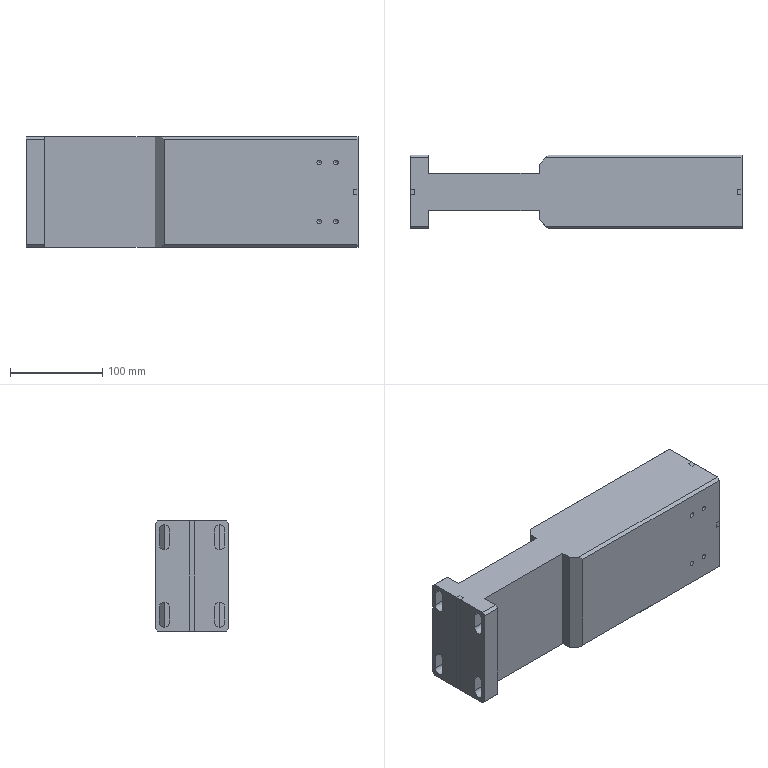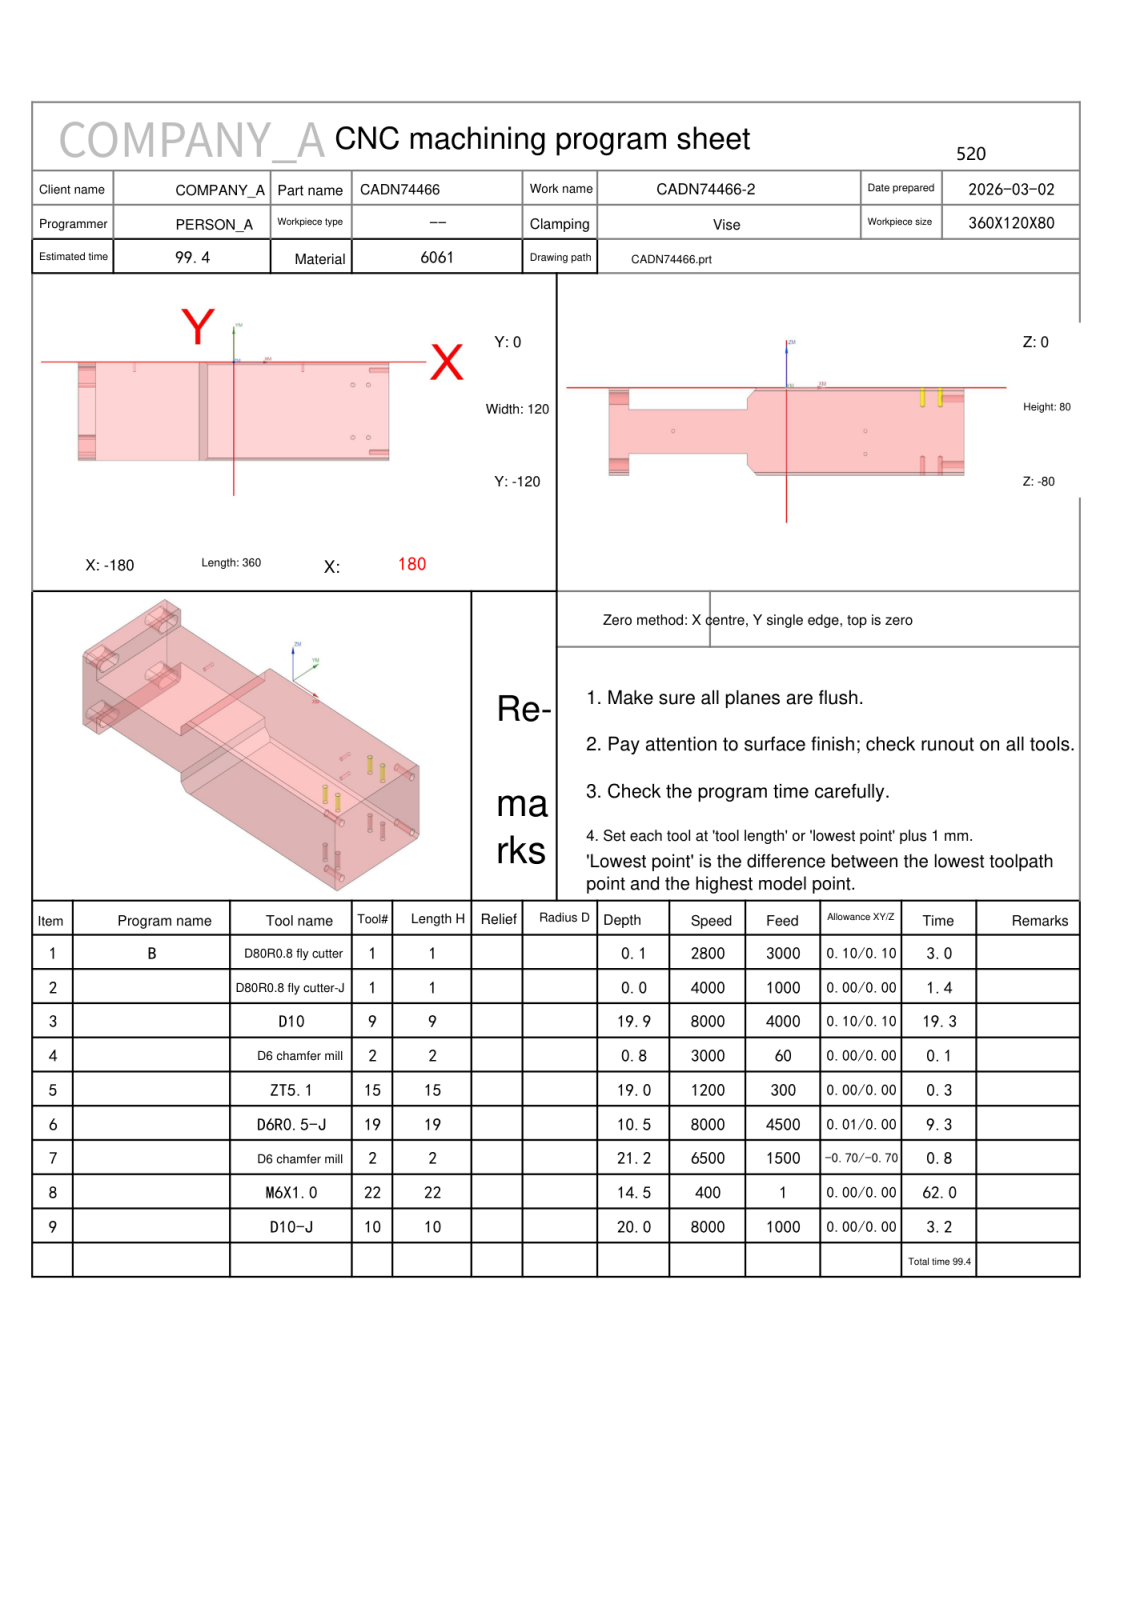NC program | NX | posted by the shop | part box 360 x 80 x 120 mm
Lines 151 to 1257 of 6245:
N3 T09 M06
(D10  D=10. R=0. H=09 ce=0.10 di=0.10)
G00 G90 G54 X-88.313 Y-134.5 M03 S8000
G43 H09 Z14.5
M08
Z.615
G01 Z-.585 F4000.
Y-127.08
G03 X-95.313 Y-120.08 I-7. J0.0
G01 X-147.9
X-154.698
X-154.901 Y-120.079
X-154.985 Y-120.083
X-154.98 Y-119.999
X-154.981 Y-118.512
G03 X-154.9 Y-117.606 I-5.04 J.906
G01 Y-117.585
Y-2.415
Y-2.394
G03 X-154.981 Y-1.488 I-5.121 J0.0
G01 X-154.98 Y-.001
X-154.985 Y.083
X-154.901 Y.079
X-154.697 Y.08
X-45.904
X-45.012
X-38.07
X-38.014 Y.056
X-35.725 Y-2.232
X-35.727 Y-6.92
Y-113.08
X-35.725 Y-117.768
X-38.014 Y-120.056
X-38.07 Y-120.08
X-42.727
X-45.088
X-45.904
X-92.299
G02 X-93.112 Y-119.662 I.001 J1.
G01 X-97.515 Y-113.498
G03 X-98.327 Y-113.08 I-.813 J-.582
G01 X-146.902
G02 X-147.9 Y-112.082 I.002 J1.
G01 Y-7.918
G02 X-146.902 Y-6.92 I1. J-.002
G01 X-45.904
X-45.014
X-43.724
G02 X-42.727 Y-7.918 I-.002 J-1.
G01 Y-112.082
G02 X-43.724 Y-113.08 I-1. J.002
G01 X-45.076
X-45.905
X-92.299
G02 X-93.112 Y-112.662 I.001 J1.
G01 X-97.515 Y-106.498
G03 X-98.328 Y-106.08 I-.813 J-.582
G01 X-139.903
G02 X-140.9 Y-105.083 I.003 J1.
G01 Y-14.917
G02 X-139.903 Y-13.92 I1. J-.003
G01 X-50.724
G02 X-49.727 Y-14.917 I-.003 J-1.
G01 Y-105.083
G02 X-50.724 Y-106.08 I-1. J.003
G01 X-92.299
G02 X-93.112 Y-105.662 I.001 J1.
G01 X-97.515 Y-99.498
G03 X-98.328 Y-99.08 I-.813 J-.582
G01 X-132.903
G02 X-133.9 Y-98.083 I.003 J1.
G01 Y-21.917
G02 X-132.903 Y-20.92 I1. J-.003
G01 X-57.724
G02 X-56.727 Y-21.917 I-.003 J-1.
G01 Y-98.083
G02 X-57.724 Y-99.08 I-1. J.003
G01 X-92.299
G02 X-93.112 Y-98.662 I0.0 J1.
G01 X-97.514 Y-92.498
G03 X-98.328 Y-92.08 I-.813 J-.582
G01 X-125.903
G02 X-126.9 Y-91.083 I.003 J1.
G01 Y-28.917
G02 X-125.903 Y-27.92 I1. J-.003
G01 X-64.723
G02 X-63.727 Y-28.917 I-.003 J-1.
G01 Y-91.083
G02 X-64.723 Y-92.08 I-1. J.003
G01 X-92.299
G02 X-93.112 Y-91.662 I0.0 J1.
G01 X-97.514 Y-85.498
G03 X-98.328 Y-85.08 I-.814 J-.582
G01 X-118.904
G02 X-119.9 Y-84.084 I.004 J1.
G01 Y-35.916
G02 X-118.904 Y-34.92 I1. J-.004
G01 X-71.723
G02 X-70.727 Y-35.916 I-.004 J-1.
G01 Y-84.084
G02 X-71.723 Y-85.08 I-1. J.004
G01 X-92.299
G02 X-93.112 Y-84.662 I0.0 J1.
G01 X-97.514 Y-78.498
G03 X-98.328 Y-78.08 I-.814 J-.582
G01 X-111.904
G02 X-112.9 Y-77.084 I.004 J1.
G01 Y-42.916
G02 X-111.904 Y-41.92 I1. J-.004
G01 X-78.723
G02 X-77.727 Y-42.916 I-.004 J-1.
G01 Y-77.084
G02 X-78.723 Y-78.08 I-1. J.004
G01 X-92.299
G02 X-93.112 Y-77.662 I0.0 J1.
G01 X-97.514 Y-71.498
G03 X-98.328 Y-71.08 I-.814 J-.582
G01 X-104.904
G02 X-105.9 Y-70.084 I.004 J1.
G01 Y-49.916
G02 X-104.904 Y-48.92 I1. J-.004
G01 X-85.723
G02 X-84.727 Y-49.916 I-.004 J-1.
G01 Y-70.084
G02 X-85.723 Y-71.08 I-1. J.004
G01 X-92.299
G02 X-93.112 Y-70.662 I0.0 J1.
G01 X-97.554 Y-64.443
G03 X-98.134 Y-64.052 I-.814 J-.582
G02 X-98.9 Y-63.084 I.234 J.972
G01 Y-56.916
G02 X-97.904 Y-55.92 I1. J-.004
G01 X-92.723
G02 X-91.727 Y-56.916 I-.004 J-1.
G01 Y-63.084
G02 X-92.723 Y-64.08 I-1. J.004
G01 X-95.313
X-95.813
G03 X-102.813 Y-71.08 I0.0 J-7.
G01 Z.615
G00 Z3.
G01 X-88.313 Y-134.5 F6000.
G00 Z.029
G01 Z-1.171 F4000.
Y-127.08
G03 X-95.313 Y-120.08 I-7. J0.0
G01 X-147.9
X-154.698
X-154.901 Y-120.079
X-154.985 Y-120.083
X-154.98 Y-119.999
X-154.981 Y-119.07
G03 X-154.9 Y-118.171 I-5.069 J.907
G01 Y-1.829
G03 X-154.981 Y-.929 I-5.148 J-.007
G01 X-154.98 Y-.001
X-154.985 Y.083
X-154.901 Y.079
X-154.697 Y.08
X-45.904
X-45.012
X-38.07
X-38.014 Y.056
X-36.311 Y-1.646
X-36.312 Y-6.92
Y-113.08
X-36.311 Y-118.354
X-38.014 Y-120.056
X-38.07 Y-120.08
X-43.312
X-45.088
X-45.904
X-92.299
G02 X-93.112 Y-119.662 I.001 J1.
G01 X-97.515 Y-113.498
G03 X-98.327 Y-113.08 I-.813 J-.582
G01 X-146.903
G02 X-147.9 Y-112.083 I.003 J1.
G01 Y-7.917
G02 X-146.903 Y-6.92 I1. J-.003
G01 X-45.904
X-45.014
X-44.309
G02 X-43.312 Y-7.918 I-.003 J-1.
G01 Y-112.082
G02 X-44.309 Y-113.08 I-1. J.003
G01 X-45.076
X-45.905
X-92.299
G02 X-93.112 Y-112.662 I.001 J1.
G01 X-97.515 Y-106.498
G03 X-98.328 Y-106.08 I-.813 J-.582
G01 X-139.903
G02 X-140.9 Y-105.083 I.003 J1.
G01 Y-14.917
G02 X-139.903 Y-13.92 I1. J-.003
G01 X-51.309
G02 X-50.312 Y-14.917 I-.003 J-1.
G01 Y-105.083
G02 X-51.309 Y-106.08 I-1. J.003
G01 X-92.299
G02 X-93.112 Y-105.662 I.001 J1.
G01 X-97.515 Y-99.498
G03 X-98.328 Y-99.08 I-.813 J-.582
G01 X-132.903
G02 X-133.9 Y-98.083 I.003 J1.
G01 Y-21.917
G02 X-132.903 Y-20.92 I1. J-.003
G01 X-58.309
G02 X-57.312 Y-21.917 I-.003 J-1.
G01 Y-98.083
G02 X-58.309 Y-99.08 I-1. J.003
G01 X-92.299
G02 X-93.112 Y-98.662 I0.0 J1.
G01 X-97.515 Y-92.498
G03 X-98.328 Y-92.08 I-.813 J-.582
G01 X-125.904
G02 X-126.9 Y-91.084 I.004 J1.
G01 Y-28.916
G02 X-125.904 Y-27.92 I1. J-.004
G01 X-65.308
G02 X-64.312 Y-28.916 I-.004 J-1.
G01 Y-91.084
G02 X-65.308 Y-92.08 I-1. J.004
G01 X-92.299
G02 X-93.112 Y-91.662 I0.0 J1.
G01 X-97.514 Y-85.498
G03 X-98.328 Y-85.08 I-.814 J-.582
G01 X-118.904
G02 X-119.9 Y-84.084 I.004 J1.
G01 Y-35.916
G02 X-118.904 Y-34.92 I1. J-.004
G01 X-72.308
G02 X-71.312 Y-35.916 I-.004 J-1.
G01 Y-84.084
G02 X-72.308 Y-85.08 I-1. J.004
G01 X-92.299
G02 X-93.112 Y-84.662 I0.0 J1.
G01 X-97.514 Y-78.498
G03 X-98.328 Y-78.08 I-.814 J-.582
G01 X-111.904
G02 X-112.9 Y-77.084 I.004 J1.
G01 Y-42.916
G02 X-111.904 Y-41.92 I1. J-.004
G01 X-79.308
G02 X-78.312 Y-42.916 I-.004 J-1.
G01 Y-77.084
G02 X-79.308 Y-78.08 I-1. J.004
G01 X-92.299
G02 X-93.112 Y-77.662 I0.0 J1.
G01 X-97.514 Y-71.499
G03 X-98.328 Y-71.08 I-.814 J-.581
G01 X-104.904
G02 X-105.9 Y-70.084 I.004 J1.
G01 Y-49.916
G02 X-104.904 Y-48.92 I1. J-.004
G01 X-86.308
G02 X-85.312 Y-49.916 I-.004 J-1.
G01 Y-70.084
G02 X-86.308 Y-71.08 I-1. J.004
G01 X-92.299
G02 X-93.112 Y-70.661 I0.0 J1.
G01 X-97.554 Y-64.443
G03 X-98.134 Y-64.052 I-.814 J-.582
G02 X-98.9 Y-63.084 I.234 J.972
G01 Y-56.916
G02 X-97.904 Y-55.92 I1. J-.004
G01 X-93.308
G02 X-92.312 Y-56.916 I-.004 J-1.
G01 Y-63.084
G02 X-93.308 Y-64.08 I-1. J.004
G01 X-95.313
X-95.813
G03 X-102.813 Y-71.08 I0.0 J-7.
G01 Z.029
G00 Z3.
G01 X-88.313 Y-134.5 F6000.
G00 Z-.556
G01 Z-1.756 F4000.
Y-127.08
G03 X-95.313 Y-120.08 I-7. J0.0
G01 X-147.9
X-154.698
X-154.901 Y-120.079
X-154.985 Y-120.083
X-154.98 Y-119.999
Y-119.655
G03 X-154.9 Y-118.756 I-5.068 J.906
G01 Y-1.244
Y-1.223
G03 X-154.98 Y-.32 I-5.121 J0.0
G01 Y-.001
X-154.985 Y.083
X-154.901 Y.079
X-154.697 Y.08
X-45.904
X-45.012
X-38.07
X-38.014 Y.056
X-36.896 Y-1.061
X-36.897 Y-6.92
Y-113.08
X-36.896 Y-118.939
X-38.014 Y-120.056
X-38.07 Y-120.08
X-43.897
X-45.088
X-45.904
X-92.299
G02 X-93.112 Y-119.662 I.001 J1.
G01 X-97.515 Y-113.498
G03 X-98.327 Y-113.08 I-.813 J-.582
G01 X-146.903
G02 X-147.9 Y-112.083 I.003 J1.
G01 Y-7.917
G02 X-146.903 Y-6.92 I1. J-.003
G01 X-45.904
X-44.894
G02 X-43.897 Y-7.917 I-.003 J-1.
G01 Y-112.083
G02 X-44.894 Y-113.08 I-1. J.003
G01 X-45.076
X-45.905
X-92.299
G02 X-93.112 Y-112.662 I.001 J1.
G01 X-97.515 Y-106.498
G03 X-98.328 Y-106.08 I-.813 J-.582
G01 X-139.903
G02 X-140.9 Y-105.083 I.003 J1.
G01 Y-14.917
G02 X-139.903 Y-13.92 I1. J-.003
G01 X-51.894
G02 X-50.897 Y-14.917 I-.003 J-1.
G01 Y-105.083
G02 X-51.894 Y-106.08 I-1. J.003
G01 X-92.299
G02 X-93.112 Y-105.662 I.001 J1.
G01 X-97.515 Y-99.498
G03 X-98.328 Y-99.08 I-.813 J-.582
G01 X-132.904
G02 X-133.9 Y-98.084 I.004 J1.
G01 Y-21.916
G02 X-132.904 Y-20.92 I1. J-.004
G01 X-58.894
G02 X-57.897 Y-21.916 I-.004 J-1.
G01 Y-98.084
G02 X-58.894 Y-99.08 I-1. J.004
G01 X-92.299
G02 X-93.112 Y-98.662 I0.0 J1.
G01 X-97.514 Y-92.498
G03 X-98.328 Y-92.08 I-.813 J-.582
G01 X-125.904
G02 X-126.9 Y-91.084 I.004 J1.
G01 Y-28.916
G02 X-125.904 Y-27.92 I1. J-.004
G01 X-65.894
G02 X-64.897 Y-28.916 I-.004 J-1.
G01 Y-91.084
G02 X-65.894 Y-92.08 I-1. J.004
G01 X-92.299
G02 X-93.112 Y-91.662 I0.0 J1.
G01 X-97.514 Y-85.498
G03 X-98.328 Y-85.08 I-.814 J-.582
G01 X-118.904
G02 X-119.9 Y-84.084 I.004 J1.
G01 Y-35.916
G02 X-118.904 Y-34.92 I1. J-.004
G01 X-72.893
G02 X-71.897 Y-35.916 I-.004 J-1.
G01 Y-84.084
G02 X-72.893 Y-85.08 I-1. J.004
G01 X-92.299
G02 X-93.112 Y-84.662 I0.0 J1.
G01 X-97.514 Y-78.498
G03 X-98.328 Y-78.08 I-.814 J-.582
G01 X-111.904
G02 X-112.9 Y-77.084 I.004 J1.
G01 Y-42.916
G02 X-111.904 Y-41.92 I1. J-.004
G01 X-79.893
G02 X-78.897 Y-42.916 I-.004 J-1.
G01 Y-77.084
G02 X-79.893 Y-78.08 I-1. J.004
G01 X-92.299
G02 X-93.112 Y-77.662 I0.0 J1.
G01 X-97.514 Y-71.498
G03 X-98.328 Y-71.08 I-.814 J-.582
G01 X-104.904
G02 X-105.9 Y-70.084 I.004 J1.
G01 Y-49.916
G02 X-104.904 Y-48.92 I1. J-.004
G01 X-86.893
G02 X-85.897 Y-49.916 I-.004 J-1.
G01 Y-70.084
G02 X-86.893 Y-71.08 I-1. J.004
G01 X-92.299
G02 X-93.112 Y-70.661 I0.0 J1.
G01 X-97.554 Y-64.443
G03 X-98.134 Y-64.052 I-.814 J-.582
G02 X-98.9 Y-63.084 I.234 J.972
G01 Y-56.916
G02 X-97.904 Y-55.92 I1. J-.004
G01 X-93.893
G02 X-92.897 Y-56.916 I-.004 J-1.
G01 Y-63.084
G02 X-93.893 Y-64.08 I-1. J.004
G01 X-95.313
X-95.813
G03 X-102.813 Y-71.08 I0.0 J-7.
G01 Z-.556
G00 Z3.
G01 X-88.313 Y-134.5 F6000.
G00 Z-1.141
G01 Z-2.341 F4000.
Y-127.08
G03 X-95.313 Y-120.08 I-7. J0.0
G01 X-147.9
X-154.698
X-154.901 Y-120.079
X-154.952 Y-120.06
G03 X-154.9 Y-119.341 I-5.099 J.728
G01 Y-.659
G03 X-154.952 Y.06 I-5.151 J-.009
G01 X-154.901 Y.079
X-154.697 Y.08
X-45.904
X-45.012
X-38.07
X-38.014 Y.056
X-37.481 Y-.476
X-37.483 Y-6.92
Y-113.076
X-37.481 Y-119.524
X-38.014 Y-120.056
X-38.07 Y-120.08
X-44.483
X-45.088
X-45.904
X-92.299
G02 X-93.112 Y-119.662 I.001 J1.
G01 X-97.515 Y-113.498
G03 X-98.327 Y-113.08 I-.813 J-.582
G01 X-146.903
G02 X-147.9 Y-112.083 I.003 J1.
G01 Y-7.917
G02 X-146.903 Y-6.92 I1. J-.003
G01 X-45.904
X-45.479
G02 X-44.483 Y-7.917 I-.003 J-1.
G01 Y-112.083
G02 X-45.479 Y-113.08 I-1. J.003
G01 X-45.905
X-92.299
G02 X-93.112 Y-112.662 I.001 J1.
G01 X-97.515 Y-106.498
G03 X-98.328 Y-106.08 I-.813 J-.582
G01 X-139.903
G02 X-140.9 Y-105.083 I.003 J1.
G01 Y-14.917
G02 X-139.903 Y-13.92 I1. J-.003
G01 X-52.479
G02 X-51.483 Y-14.917 I-.003 J-1.
G01 Y-105.083
G02 X-52.479 Y-106.08 I-1. J.003
G01 X-92.299
G02 X-93.112 Y-105.662 I.001 J1.
G01 X-97.514 Y-99.498
G03 X-98.328 Y-99.08 I-.813 J-.582
G01 X-132.904
G02 X-133.9 Y-98.084 I.004 J1.
G01 Y-21.916
G02 X-132.904 Y-20.92 I1. J-.004
G01 X-59.479
G02 X-58.483 Y-21.916 I-.004 J-1.
G01 Y-98.084
G02 X-59.479 Y-99.08 I-1. J.004
G01 X-92.299
G02 X-93.112 Y-98.662 I0.0 J1.
G01 X-97.514 Y-92.498
G03 X-98.328 Y-92.08 I-.813 J-.582
G01 X-125.904
G02 X-126.9 Y-91.084 I.004 J1.
G01 Y-28.916
G02 X-125.904 Y-27.92 I1. J-.004
G01 X-66.479
G02 X-65.483 Y-28.916 I-.004 J-1.
G01 Y-91.084
G02 X-66.479 Y-92.08 I-1. J.004
G01 X-92.299
G02 X-93.112 Y-91.662 I0.0 J1.
G01 X-97.514 Y-85.498
G03 X-98.328 Y-85.08 I-.813 J-.582
G01 X-118.904
G02 X-119.9 Y-84.084 I.004 J1.
G01 Y-35.916
G02 X-118.904 Y-34.92 I1. J-.004
G01 X-73.478
G02 X-72.483 Y-35.916 I-.004 J-1.
G01 Y-84.084
G02 X-73.478 Y-85.08 I-1. J.004
G01 X-92.299
G02 X-93.112 Y-84.662 I0.0 J1.
G01 X-97.514 Y-78.498
G03 X-98.328 Y-78.08 I-.814 J-.582
G01 X-111.904
G02 X-112.9 Y-77.084 I.004 J1.
G01 Y-42.916
G02 X-111.904 Y-41.92 I1. J-.004
G01 X-80.478
G02 X-79.483 Y-42.916 I-.004 J-1.
G01 Y-77.084
G02 X-80.478 Y-78.08 I-1. J.004
G01 X-92.299
G02 X-93.112 Y-77.662 I0.0 J1.
G01 X-97.514 Y-71.499
G03 X-98.328 Y-71.08 I-.814 J-.581
G01 X-104.904
G02 X-105.9 Y-70.084 I.004 J1.
G01 Y-49.916
G02 X-104.904 Y-48.92 I1. J-.004
G01 X-87.478
G02 X-86.483 Y-49.916 I-.004 J-1.
G01 Y-70.084
G02 X-87.478 Y-71.08 I-1. J.004
G01 X-92.299
G02 X-93.112 Y-70.661 I0.0 J1.
G01 X-97.554 Y-64.443
G03 X-98.134 Y-64.052 I-.814 J-.582
G02 X-98.9 Y-63.084 I.234 J.972
G01 Y-56.916
G02 X-97.904 Y-55.92 I1. J-.004
G01 X-94.478
G02 X-93.483 Y-56.916 I-.004 J-1.
G01 Y-63.084
G02 X-94.478 Y-64.08 I-1. J.004
G01 X-95.313
X-95.813
G03 X-102.813 Y-71.08 I0.0 J-7.
G01 Z-1.141
G00 Z3.
G01 X-88.313 Y-134.5 F6000.
G00 Z-1.726
G01 Z-2.926 F4000.
Y-127.08
G03 X-95.313 Y-120.08 I-7. J0.0
G01 X-147.9
X-154.698
X-154.902 Y-120.079
X-154.9 Y-119.926
Y-.074
X-154.902 Y.079
X-154.697 Y.08
X-45.904
X-45.012
X-38.067
X-38.068 Y-.062
Y-119.938
X-38.067 Y-120.08
X-45.088
X-45.904
X-92.299
G02 X-93.112 Y-119.662 I.001 J1.
G01 X-97.515 Y-113.498
G03 X-98.327 Y-113.08 I-.813 J-.582
G01 X-146.903
G02 X-147.9 Y-112.083 I.003 J1.
G01 Y-7.917
G02 X-146.903 Y-6.92 I1. J-.003
G01 X-46.065
G02 X-45.068 Y-7.917 I-.003 J-1.
G01 Y-112.083
G02 X-46.065 Y-113.08 I-1. J.003
G01 X-92.299
G02 X-93.112 Y-112.662 I.001 J1.
G01 X-97.515 Y-106.498
G03 X-98.328 Y-106.08 I-.813 J-.582
G01 X-139.904
G02 X-140.9 Y-105.084 I.004 J1.
G01 Y-14.916
G02 X-139.904 Y-13.92 I1. J-.004
G01 X-53.064
G02 X-52.068 Y-14.916 I-.004 J-1.
G01 Y-105.084
G02 X-53.064 Y-106.08 I-1. J.004
G01 X-92.299
G02 X-93.112 Y-105.662 I.001 J1.
G01 X-97.515 Y-99.498
G03 X-98.328 Y-99.08 I-.813 J-.582
G01 X-132.904
G02 X-133.9 Y-98.084 I.004 J1.
G01 Y-21.916
G02 X-132.904 Y-20.92 I1. J-.004
G01 X-60.064
G02 X-59.068 Y-21.916 I-.004 J-1.
G01 Y-98.084
G02 X-60.064 Y-99.08 I-1. J.004
G01 X-92.299
G02 X-93.112 Y-98.662 I0.0 J1.
G01 X-97.514 Y-92.498
G03 X-98.328 Y-92.08 I-.813 J-.582
G01 X-125.904
G02 X-126.9 Y-91.084 I.004 J1.
G01 Y-28.916
G02 X-125.904 Y-27.92 I1. J-.004
G01 X-67.064
G02 X-66.068 Y-28.916 I-.004 J-1.
G01 Y-91.084
G02 X-67.064 Y-92.08 I-1. J.004
G01 X-92.299
G02 X-93.112 Y-91.662 I0.0 J1.
G01 X-97.514 Y-85.498
G03 X-98.328 Y-85.08 I-.813 J-.582
G01 X-118.904
G02 X-119.9 Y-84.084 I.004 J1.
G01 Y-35.916
G02 X-118.904 Y-34.92 I1. J-.004
G01 X-74.064
G02 X-73.068 Y-35.916 I-.004 J-1.
G01 Y-84.084
G02 X-74.064 Y-85.08 I-1. J.004
G01 X-92.299
G02 X-93.112 Y-84.662 I0.0 J1.
G01 X-97.514 Y-78.498
G03 X-98.328 Y-78.08 I-.814 J-.582
G01 X-111.904
G02 X-112.9 Y-77.084 I.004 J1.
G01 Y-42.916
G02 X-111.904 Y-41.92 I1. J-.004
G01 X-81.063
G02 X-80.068 Y-42.916 I-.004 J-1.
G01 Y-77.084
G02 X-81.063 Y-78.08 I-1. J.004
G01 X-92.299
G02 X-93.112 Y-77.662 I0.0 J1.
G01 X-97.514 Y-71.499
G03 X-98.328 Y-71.08 I-.814 J-.581
G01 X-104.905
G02 X-105.9 Y-70.085 I.005 J1.
G01 Y-49.915
G02 X-104.905 Y-48.92 I1. J-.005
G01 X-88.063
G02 X-87.068 Y-49.915 I-.005 J-1.
G01 Y-70.085
G02 X-88.063 Y-71.08 I-1. J.005
G01 X-92.299
G02 X-93.112 Y-70.661 I0.0 J1.
G01 X-97.554 Y-64.443
G03 X-98.134 Y-64.052 I-.814 J-.582
G02 X-98.9 Y-63.085 I.234 J.972
G01 Y-56.915
G02 X-97.905 Y-55.92 I1. J-.005
G01 X-95.063
G02 X-94.068 Y-56.915 I-.005 J-1.
G01 Y-63.085
G02 X-95.063 Y-64.08 I-1. J.005
G01 X-95.313
X-95.813
G03 X-102.813 Y-71.08 I0.0 J-7.
G01 Z-1.726
G00 Z3.
G01 X-88.313 Y-134.5 F6000.
G00 Z-2.312
G01 Z-3.512 F4000.
Y-127.08
G03 X-95.313 Y-120.08 I-7. J0.0
G01 X-147.9
X-154.698
X-154.901 Y-120.079
X-154.9 Y-119.927
X-154.901 Y.079
X-154.697 Y.08
X-45.904
X-45.653
X-45.012
X-38.652
X-38.653 Y-6.92
Y-113.08
X-38.652 Y-120.08
X-45.088
X-45.904
X-92.299
G02 X-93.112 Y-119.662 I.001 J1.
G01 X-97.515 Y-113.498
G03 X-98.327 Y-113.08 I-.813 J-.582
G01 X-146.904
G02 X-147.9 Y-112.084 I.004 J1.
G01 Y-7.916
G02 X-146.904 Y-6.92 I1. J-.004
G01 X-46.65
G02 X-45.653 Y-7.916 I-.004 J-1.
G01 Y-112.084
G02 X-46.65 Y-113.08 I-1. J.004
G01 X-92.299
G02 X-93.112 Y-112.662 I.001 J1.
G01 X-97.515 Y-106.498
G03 X-98.327 Y-106.08 I-.813 J-.582
G01 X-139.904
G02 X-140.9 Y-105.084 I.004 J1.
G01 Y-14.916
G02 X-139.904 Y-13.92 I1. J-.004
G01 X-53.649
G02 X-52.653 Y-14.916 I-.004 J-1.
G01 Y-105.084
G02 X-53.649 Y-106.08 I-1. J.004
G01 X-92.299
G02 X-93.112 Y-105.662 I0.0 J1.
G01 X-97.515 Y-99.498
G03 X-98.328 Y-99.08 I-.813 J-.582
G01 X-132.904
G02 X-133.9 Y-98.084 I.004 J1.
G01 Y-21.916
G02 X-132.904 Y-20.92 I1. J-.004
G01 X-60.649
G02 X-59.653 Y-21.916 I-.004 J-1.
G01 Y-98.084
G02 X-60.649 Y-99.08 I-1. J.004
G01 X-92.299
G02 X-93.112 Y-98.662 I0.0 J1.
G01 X-97.515 Y-92.498
G03 X-98.328 Y-92.08 I-.813 J-.582
G01 X-125.904
G02 X-126.9 Y-91.084 I.004 J1.
G01 Y-28.916
G02 X-125.904 Y-27.92 I1. J-.004
G01 X-67.649
G02 X-66.653 Y-28.916 I-.004 J-1.
G01 Y-91.084
G02 X-67.649 Y-92.08 I-1. J.004
G01 X-92.299
G02 X-93.112 Y-91.662 I0.0 J1.
G01 X-97.514 Y-85.498
G03 X-98.328 Y-85.08 I-.814 J-.582
G01 X-118.904
G02 X-119.9 Y-84.084 I.004 J1.
G01 Y-35.916
G02 X-118.904 Y-34.92 I1. J-.004
G01 X-74.649
G02 X-73.653 Y-35.916 I-.004 J-1.
G01 Y-84.084
G02 X-74.649 Y-85.08 I-1. J.004
G01 X-92.299
G02 X-93.112 Y-84.662 I0.0 J1.
G01 X-97.514 Y-78.498
G03 X-98.328 Y-78.08 I-.814 J-.582
G01 X-111.905
G02 X-112.9 Y-77.085 I.005 J1.
G01 Y-42.915
G02 X-111.905 Y-41.92 I1. J-.005
G01 X-81.649
G02 X-80.653 Y-42.915 I-.005 J-1.
G01 Y-77.085
G02 X-81.649 Y-78.08 I-1. J.005
G01 X-92.299
G02 X-93.112 Y-77.662 I0.0 J1.
G01 X-97.514 Y-71.499
G03 X-98.328 Y-71.08 I-.814 J-.581
G01 X-104.905
G02 X-105.9 Y-70.085 I.005 J1.
G01 Y-49.915
G02 X-104.905 Y-48.92 I1. J-.005
G01 X-88.648
G02 X-87.653 Y-49.915 I-.005 J-1.
G01 Y-70.085
G02 X-88.648 Y-71.08 I-1. J.005
G01 X-92.315
G02 X-93.113 Y-70.682 I0.0 J1.
G01 X-97.927 Y-64.299
G03 X-98.312 Y-63.991 I-.798 J-.602
G02 X-98.9 Y-63.085 I.412 J.911
G01 Y-56.915
G02 X-97.905 Y-55.92 I1. J-.005
G01 X-95.648
G02 X-94.653 Y-56.915 I-.005 J-1.
G01 Y-63.085
G02 X-95.611 Y-64.079 I-1. J.005
G01 X-96.111 Y-64.08
G03 X-103.111 Y-71.08 I0.0 J-7.
G01 Z-2.312
G00 Z3.
G01 X-88.313 Y-134.5 F6000.
G00 Z-2.897
G01 Z-4.097 F4000.
Y-127.08
G03 X-95.313 Y-120.08 I-7. J0.0
G01 X-147.9
X-154.698
X-154.901 Y-120.079
X-154.9 Y-119.927
X-154.901 Y.079
X-154.697 Y.08
X-45.904
X-45.012
X-39.237
X-39.238 Y-6.92
Y-113.08
X-39.237 Y-120.08
X-45.088
X-45.904
X-92.299
G02 X-93.112 Y-119.662 I.001 J1.
G01 X-97.515 Y-113.498
G03 X-98.327 Y-113.08 I-.813 J-.582
G01 X-146.904
G02 X-147.9 Y-112.084 I.004 J1.
G01 Y-7.916
G02 X-146.904 Y-6.92 I1. J-.004
G01 X-47.235
G02 X-46.238 Y-7.916 I-.004 J-1.
G01 Y-112.084
G02 X-47.235 Y-113.08 I-1. J.004
G01 X-92.299
G02 X-93.112 Y-112.662 I.001 J1.
G01 X-97.515 Y-106.498
G03 X-98.328 Y-106.08 I-.813 J-.582
G01 X-139.904
G02 X-140.9 Y-105.084 I.004 J1.
G01 Y-14.916
G02 X-139.904 Y-13.92 I1. J-.004
G01 X-54.234
G02 X-53.238 Y-14.916 I-.004 J-1.
G01 Y-105.084
G02 X-54.234 Y-106.08 I-1. J.004
G01 X-92.299
G02 X-93.112 Y-105.662 I0.0 J1.
G01 X-97.515 Y-99.498
G03 X-98.328 Y-99.08 I-.813 J-.582
G01 X-132.904
G02 X-133.9 Y-98.084 I.004 J1.
G01 Y-21.916
G02 X-132.904 Y-20.92 I1. J-.004
G01 X-61.234
G02 X-60.238 Y-21.916 I-.004 J-1.
G01 Y-98.084
G02 X-61.234 Y-99.08 I-1. J.004
G01 X-92.299
G02 X-93.112 Y-98.662 I0.0 J1.
G01 X-97.514 Y-92.498
G03 X-98.328 Y-92.08 I-.813 J-.582
G01 X-125.904
G02 X-126.9 Y-91.085 I.004 J1.
G01 Y-28.916
G02 X-125.904 Y-27.92 I1. J-.004
G01 X-68.234
G02 X-67.238 Y-28.916 I-.004 J-1.
G01 Y-91.084
G02 X-68.234 Y-92.08 I-1. J.004
G01 X-92.299
G02 X-93.112 Y-91.662 I0.0 J1.
G01 X-97.514 Y-85.498
G03 X-98.328 Y-85.08 I-.813 J-.582
G01 X-118.905
G02 X-119.9 Y-84.085 I.005 J1.
G01 Y-35.915
G02 X-118.905 Y-34.92 I1. J-.005
G01 X-75.234
G02 X-74.238 Y-35.915 I-.005 J-1.
G01 Y-84.085
G02 X-75.234 Y-85.08 I-1. J.005
G01 X-92.299
G02 X-93.112 Y-84.662 I0.0 J1.
G01 X-97.514 Y-78.498
G03 X-98.328 Y-78.08 I-.814 J-.582
G01 X-111.905
G02 X-112.9 Y-77.085 I.005 J1.
G01 Y-42.915
G02 X-111.905 Y-41.92 I1. J-.005
G01 X-82.234
G02 X-81.238 Y-42.915 I-.005 J-1.
G01 Y-77.085
G02 X-82.234 Y-78.08 I-1. J.005
G01 X-92.299
G02 X-93.112 Y-77.662 I0.0 J1.
G01 X-97.514 Y-71.499
G03 X-98.328 Y-71.08 I-.814 J-.581
G01 X-104.905
G02 X-105.9 Y-70.085 I.005 J1.
G01 Y-49.915
G02 X-104.905 Y-48.92 I1. J-.005
G01 X-89.234
G02 X-88.238 Y-49.915 I-.005 J-1.
G01 Y-70.085
G02 X-89.234 Y-71.08 I-1. J.005
G01 X-92.33
G02 X-93.113 Y-70.702 I0.0 J1.
G01 X-98.517 Y-63.887
X-98.6 Y-63.794
G02 X-98.9 Y-63.085 I.7 J.714
G01 Y-56.915
G02 X-97.905 Y-55.92 I1. J-.005
G01 X-96.234
G02 X-95.238 Y-56.915 I-.005 J-1.
G01 Y-63.085
G02 X-96.124 Y-64.073 I-1. J.005
G01 X-96.234 Y-64.08
X-96.623
G03 X-103.623 Y-71.08 I0.0 J-7.
G01 Z-2.897
G00 Z3.
G01 X-88.313 Y-134.5 F6000.
G00 Z-3.482
G01 Z-4.682 F4000.
Y-127.08
G03 X-95.313 Y-120.08 I-7. J0.0
G01 X-147.9
X-154.698
X-154.901 Y-120.079
X-154.9 Y-119.927
X-154.901 Y.079
X-154.697 Y.08
X-45.904
X-45.012
X-39.822
X-39.824 Y-6.92
Y-113.08
X-39.822 Y-120.08
X-45.088
X-45.904
X-92.299
G02 X-93.112 Y-119.662 I.001 J1.
G01 X-97.515 Y-113.498
G03 X-98.327 Y-113.08 I-.813 J-.582
G01 X-146.904
G02 X-147.9 Y-112.084 I.004 J1.
G01 Y-7.916
G02 X-146.904 Y-6.92 I1. J-.004
G01 X-47.82
G02 X-46.824 Y-7.916 I-.004 J-1.
G01 Y-112.084
G02 X-47.82 Y-113.08 I-1. J.004
G01 X-92.299
G02 X-93.112 Y-112.662 I.001 J1.
G01 X-97.515 Y-106.498
G03 X-98.327 Y-106.08 I-.813 J-.582
G01 X-139.904
G02 X-140.9 Y-105.084 I.004 J1.
G01 Y-14.916
G02 X-139.904 Y-13.92 I1. J-.004
G01 X-54.82
G02 X-53.824 Y-14.916 I-.004 J-1.
G01 Y-105.084
G02 X-54.82 Y-106.08 I-1. J.004
G01 X-92.299
G02 X-93.112 Y-105.662 I0.0 J1.
G01 X-97.515 Y-99.498
G03 X-98.328 Y-99.08 I-.813 J-.582
G01 X-132.904
G02 X-133.9 Y-98.084 I.004 J1.
G01 Y-21.916
G02 X-132.904 Y-20.92 I1. J-.004
G01 X-61.819
G02 X-60.824 Y-21.916 I-.004 J-1.
G01 Y-98.084
G02 X-61.819 Y-99.08 I-1. J.004
G01 X-92.299
G02 X-93.112 Y-98.662 I0.0 J1.
G01 X-97.514 Y-92.498
G03 X-98.328 Y-92.08 I-.813 J-.582
G01 X-125.905
G02 X-126.9 Y-91.085 I.005 J1.
G01 Y-28.915
G02 X-125.905 Y-27.92 I1. J-.005
G01 X-68.819
G02 X-67.824 Y-28.915 I-.005 J-1.
G01 Y-91.085
G02 X-68.819 Y-92.08 I-1. J.005
G01 X-92.299
G02 X-93.112 Y-91.662 I0.0 J1.
G01 X-97.514 Y-85.498
G03 X-98.328 Y-85.08 I-.814 J-.582
G01 X-118.905
G02 X-119.9 Y-84.085 I.005 J1.
G01 Y-35.915
G02 X-118.905 Y-34.92 I1. J-.005
G01 X-75.819
G02 X-74.824 Y-35.915 I-.005 J-1.
G01 Y-84.085
G02 X-75.819 Y-85.08 I-1. J.005
G01 X-92.299
G02 X-93.112 Y-84.662 I0.0 J1.
G01 X-97.514 Y-78.498
G03 X-98.328 Y-78.08 I-.814 J-.582
G01 X-111.905
G02 X-112.9 Y-77.085 I.005 J1.
G01 Y-42.915
G02 X-111.905 Y-41.92 I1. J-.005
G01 X-82.819
G02 X-81.824 Y-42.915 I-.005 J-1.
G01 Y-77.085
G02 X-82.819 Y-78.08 I-1. J.005
G01 X-92.299
G02 X-93.112 Y-77.662 I0.0 J1.
G01 X-97.514 Y-71.499
G03 X-98.328 Y-71.08 I-.814 J-.581
G01 X-104.905
G02 X-105.9 Y-70.085 I.005 J1.
G01 Y-49.915
G02 X-104.905 Y-48.92 I1. J-.005
G01 X-89.819
G02 X-88.824 Y-49.915 I-.005 J-1.
G01 Y-70.085
G02 X-89.819 Y-71.08 I-1. J.005
G01 X-92.304
G02 X-93.113 Y-70.668 I0.0 J1.
G01 X-97.667 Y-64.407
G03 X-98.188 Y-64.038 I-.808 J-.589
G02 X-98.9 Y-63.085 I.288 J.958
G01 Y-56.915
G02 X-97.905 Y-55.92 I1. J-.005
G01 X-96.819
G02 X-95.824 Y-56.915 I-.005 J-1.
G01 Y-63.085
G02 X-96.638 Y-64.063 I-1. J.005
G01 X-96.819 Y-64.08
X-97.137
G03 X-104.137 Y-71.08 I0.0 J-7.
G01 Z-3.482
G00 Z3.
G01 X-88.313 Y-134.5 F6000.
G00 Z-4.068
G01 Z-5.268 F4000.
Y-127.08
G03 X-95.313 Y-120.08 I-7. J0.0
G01 X-147.9
X-154.698
X-154.901 Y-120.079
X-154.9 Y-119.927
X-154.901 Y.079
X-154.697 Y.08
X-45.904
X-45.012
X-40.408
X-40.409 Y-6.92
Y-113.08
X-40.408 Y-120.08
X-45.088
X-45.904
X-92.299
G02 X-93.112 Y-119.662 I.001 J1.
G01 X-97.515 Y-113.498
G03 X-98.327 Y-113.08 I-.813 J-.582
G01 X-146.904
G02 X-147.9 Y-112.084 I.004 J1.
G01 Y-7.916
G02 X-146.904 Y-6.92 I1. J-.004
G01 X-48.405
G02 X-47.409 Y-7.916 I-.004 J-1.
G01 Y-112.084
G02 X-48.405 Y-113.08 I-1. J.004
G01 X-92.299
G02 X-93.112 Y-112.662 I.001 J1.
G01 X-97.515 Y-106.498
G03 X-98.328 Y-106.08 I-.813 J-.582
G01 X-139.904
G02 X-140.9 Y-105.084 I.004 J1.
G01 Y-14.916
G02 X-139.904 Y-13.92 I1. J-.004
G01 X-55.405
G02 X-54.409 Y-14.916 I-.004 J-1.
G01 Y-105.084
G02 X-55.405 Y-106.08 I-1. J.004
G01 X-92.299
G02 X-93.112 Y-105.662 I.001 J1.
G01 X-97.515 Y-99.498
G03 X-98.328 Y-99.08 I-.813 J-.582
G01 X-132.905
G02 X-133.9 Y-98.085 I.005 J1.
G01 Y-21.915
G02 X-132.905 Y-20.92 I1. J-.005
G01 X-62.404
G02 X-61.409 Y-21.915 I-.005 J-1.
G01 Y-98.085
G02 X-62.404 Y-99.08 I-1. J.005
G01 X-92.299
G02 X-93.112 Y-98.662 I0.0 J1.
G01 X-97.515 Y-92.498
G03 X-98.328 Y-92.08 I-.813 J-.582
G01 X-125.905
G02 X-126.9 Y-91.085 I.005 J1.
G01 Y-28.915
G02 X-125.905 Y-27.92 I1. J-.005
G01 X-69.404
G02 X-68.409 Y-28.915 I-.005 J-1.
G01 Y-91.085
G02 X-69.404 Y-92.08 I-1. J.005
G01 X-92.299
G02 X-93.112 Y-91.662 I0.0 J1.
G01 X-97.514 Y-85.498
G03 X-98.328 Y-85.08 I-.814 J-.582
G01 X-118.905
G02 X-119.9 Y-84.085 I.005 J1.
G01 Y-35.915
G02 X-118.905 Y-34.92 I1. J-.005
G01 X-76.404
G02 X-75.409 Y-35.915 I-.005 J-1.
G01 Y-84.085
G02 X-76.404 Y-85.08 I-1. J.005
G01 X-92.299
G02 X-93.112 Y-84.662 I0.0 J1.
G01 X-97.514 Y-78.498
G03 X-98.328 Y-78.08 I-.814 J-.582
G01 X-111.905
G02 X-112.9 Y-77.085 I.005 J1.
G01 Y-42.915
G02 X-111.905 Y-41.92 I1. J-.005
G01 X-83.404
G02 X-82.409 Y-42.915 I-.005 J-1.
G01 Y-77.085